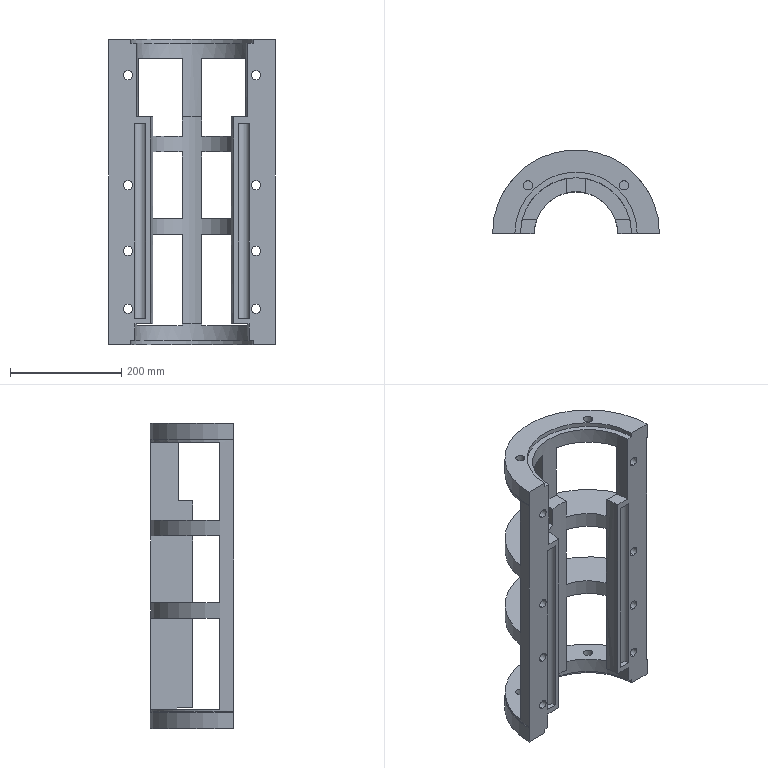Part | SolidWorks | features ICE 6, HoleWzd 3, RevCut 3, Revolution 1 | 1 solid | 76 faces | box 300 x 150 x 550 mm | volume 5053436 mm3 | plane 41 | cylinder 34 | torus 1 | commonest cylinder face diameters 16.5 x24 20.5 x2 220 x2 300 x2 150 x1 200 x1